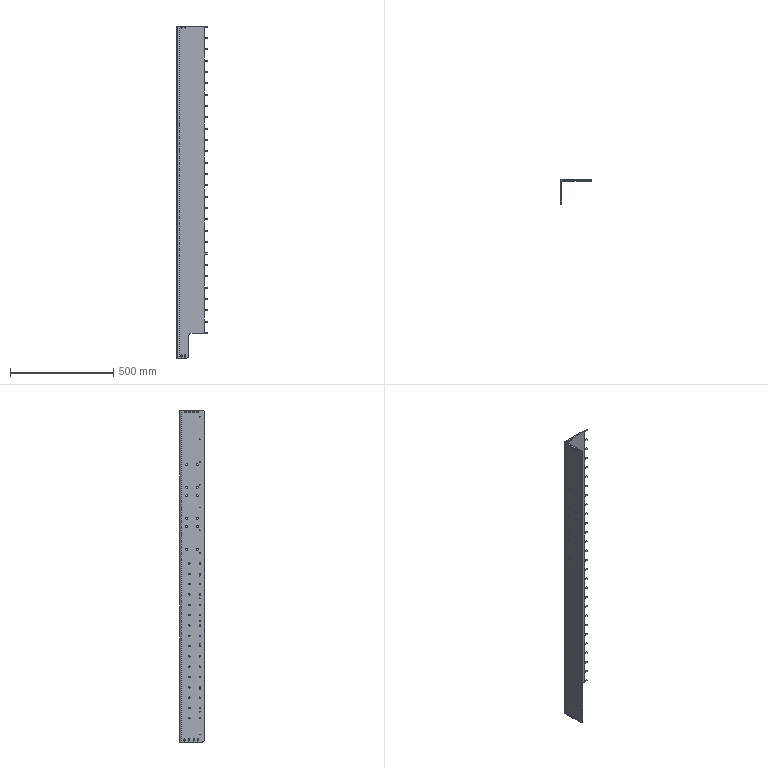Part | SolidWorks | features HoleWzd 7, Fillet 2, LPattern 2, Cut 1, Extrusion 1, ICE 1, MoveFace 1 | 1 solid | 295 faces | box 150 x 120 x 1609 mm | volume 2345426 mm3 | cylinder 153 | plane 130 | cone 12 | commonest cylinder face diameters 6.8 x63 4.2 x30 10 x24 5.8 x18 5.5 x12 20 x4